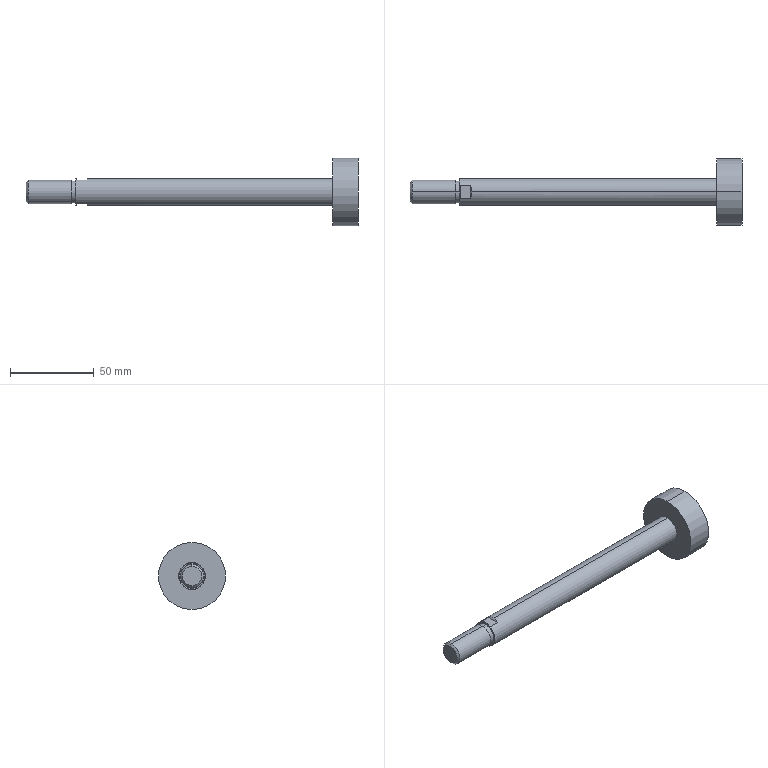Part | SolidWorks | features BaseBody 1 | 1 solid | 23 faces | box 198 x 40 x 40 mm | volume 54072 mm3 | plane 11 | cylinder 8 | cone 4 | commonest cylinder face diameters 13 x2 14 x2 16 x2 40 x2
STEP:
#1=CARTESIAN_POINT('',(133.,0.,8.));
#2=VERTEX_POINT('',#1);
#3=CARTESIAN_POINT('',(133.,0.,-8.));
#4=VERTEX_POINT('',#3);
#5=CARTESIAN_POINT('',(133.,0.,0.));
#6=DIRECTION('',(-1.,0.,0.));
#7=DIRECTION('',(0.,0.,1.));
#8=AXIS2_PLACEMENT_3D('',#5,#6,#7);
#9=CIRCLE('',#8,8.);
#10=EDGE_CURVE('',#2,#4,#9,.T.);
#11=ORIENTED_EDGE('',*,*,#10,.T.);
#12=CARTESIAN_POINT('',(-13.,0.,-8.));
#13=VERTEX_POINT('',#12);
#14=CARTESIAN_POINT('',(148.,0.,-8.));
#15=DIRECTION('',(-1.,0.,0.));
#16=VECTOR('',#15,1000.);
#17=LINE('',#14,#16);
#18=EDGE_CURVE('',#4,#13,#17,.T.);
#19=ORIENTED_EDGE('',*,*,#18,.T.);
#20=CARTESIAN_POINT('',(-14.,3.873,-7.));
#21=VERTEX_POINT('',#20);
#22=CARTESIAN_POINT('',(-13.,0.,-8.));
#23=CARTESIAN_POINT('',(-13.,1.362,-8.));
#24=CARTESIAN_POINT('',(-13.341,2.681,-7.659));
#25=CARTESIAN_POINT('',(-14.,3.873,-7.));
#26=(BOUNDED_CURVE()B_SPLINE_CURVE(3,(#22,#23,#24,#25),.UNSPECIFIED.,.F.,.F.)B_SPLINE_CURVE_WITH_KNOTS((4,4),(3.142,3.647),.UNSPECIFIED.)CURVE()GEOMETRIC_REPRESENTATION_ITEM()RATIONAL_B_SPLINE_CURVE((1.,0.9788,0.9788,1.))REPRESENTATION_ITEM(''));
#27=EDGE_CURVE('',#13,#21,#26,.T.);
#28=ORIENTED_EDGE('',*,*,#27,.T.);
#29=CARTESIAN_POINT('',(-20.,3.873,-7.));
#30=VERTEX_POINT('',#29);
#31=CARTESIAN_POINT('',(148.,3.873,-7.));
#32=DIRECTION('',(-1.,0.,0.));
#33=VECTOR('',#32,1000.);
#34=LINE('',#31,#33);
#35=EDGE_CURVE('',#21,#30,#34,.T.);
#36=ORIENTED_EDGE('',*,*,#35,.T.);
#37=CARTESIAN_POINT('',(-20.,0.,-8.));
#38=VERTEX_POINT('',#37);
#39=CARTESIAN_POINT('',(-20.,0.,0.));
#40=DIRECTION('',(-1.,0.,0.));
#41=DIRECTION('',(0.,0.,1.));
#42=AXIS2_PLACEMENT_3D('',#39,#40,#41);
#43=CIRCLE('',#42,8.);
#44=EDGE_CURVE('',#30,#38,#43,.T.);
#45=ORIENTED_EDGE('',*,*,#44,.T.);
#46=CARTESIAN_POINT('',(-20.4,0.,-8.));
#47=VERTEX_POINT('',#46);
#48=CARTESIAN_POINT('',(148.,0.,-8.));
#49=DIRECTION('',(-1.,0.,0.));
#50=VECTOR('',#49,1000.);
#51=LINE('',#48,#50);
#52=EDGE_CURVE('',#38,#47,#51,.T.);
#53=ORIENTED_EDGE('',*,*,#52,.T.);
#54=CARTESIAN_POINT('',(-20.4,0.,8.));
#55=VERTEX_POINT('',#54);
#56=CARTESIAN_POINT('',(-20.4,0.,0.));
#57=DIRECTION('',(1.,0.,0.));
#58=DIRECTION('',(0.,0.,1.));
#59=AXIS2_PLACEMENT_3D('',#56,#57,#58);
#60=CIRCLE('',#59,8.);
#61=EDGE_CURVE('',#47,#55,#60,.T.);
#62=ORIENTED_EDGE('',*,*,#61,.T.);
#63=CARTESIAN_POINT('',(-20.,0.,8.));
#64=VERTEX_POINT('',#63);
#65=CARTESIAN_POINT('',(148.,0.,8.));
#66=DIRECTION('',(-1.,0.,0.));
#67=VECTOR('',#66,1000.);
#68=LINE('',#65,#67);
#69=EDGE_CURVE('',#64,#55,#68,.T.);
#70=ORIENTED_EDGE('',*,*,#69,.F.);
#71=CARTESIAN_POINT('',(-20.,3.873,7.));
#72=VERTEX_POINT('',#71);
#73=CARTESIAN_POINT('',(-20.,0.,0.));
#74=DIRECTION('',(-1.,0.,0.));
#75=DIRECTION('',(0.,0.,1.));
#76=AXIS2_PLACEMENT_3D('',#73,#74,#75);
#77=CIRCLE('',#76,8.);
#78=EDGE_CURVE('',#64,#72,#77,.T.);
#79=ORIENTED_EDGE('',*,*,#78,.T.);
#80=CARTESIAN_POINT('',(-14.,3.873,7.));
#81=VERTEX_POINT('',#80);
#82=CARTESIAN_POINT('',(148.,3.873,7.));
#83=DIRECTION('',(1.,0.,0.));
#84=VECTOR('',#83,1000.);
#85=LINE('',#82,#84);
#86=EDGE_CURVE('',#72,#81,#85,.T.);
#87=ORIENTED_EDGE('',*,*,#86,.T.);
#88=CARTESIAN_POINT('',(-13.,0.,8.));
#89=VERTEX_POINT('',#88);
#90=CARTESIAN_POINT('',(-14.,3.873,7.));
#91=CARTESIAN_POINT('',(-13.341,2.681,7.659));
#92=CARTESIAN_POINT('',(-13.,1.362,8.));
#93=CARTESIAN_POINT('',(-13.,0.,8.));
#94=(BOUNDED_CURVE()B_SPLINE_CURVE(3,(#90,#91,#92,#93),.UNSPECIFIED.,.F.,.T.)B_SPLINE_CURVE_WITH_KNOTS((4,4),(2.636,3.142),.UNSPECIFIED.)CURVE()GEOMETRIC_REPRESENTATION_ITEM()RATIONAL_B_SPLINE_CURVE((1.,0.9788,0.9788,1.))REPRESENTATION_ITEM(''));
#95=EDGE_CURVE('',#81,#89,#94,.T.);
#96=ORIENTED_EDGE('',*,*,#95,.T.);
#97=CARTESIAN_POINT('',(148.,0.,8.));
#98=DIRECTION('',(-1.,0.,0.));
#99=VECTOR('',#98,1000.);
#100=LINE('',#97,#99);
#101=EDGE_CURVE('',#2,#89,#100,.T.);
#102=ORIENTED_EDGE('',*,*,#101,.F.);
#103=EDGE_LOOP('',(#11,#19,#28,#36,#45,#53,#62,#70,#79,#87,#96,#102));
#104=FACE_OUTER_BOUND('',#103,.T.);
#105=CARTESIAN_POINT('',(148.,0.,0.));
#106=DIRECTION('',(-1.,0.,0.));
#107=DIRECTION('',(0.,0.,1.));
#108=AXIS2_PLACEMENT_3D('',#105,#106,#107);
#109=CYLINDRICAL_SURFACE('',#108,8.);
#110=ADVANCED_FACE('',(#104),#109,.T.);
#111=CARTESIAN_POINT('',(-20.,0.,-7.6));
#112=VERTEX_POINT('',#111);
#113=CARTESIAN_POINT('',(-20.,-2.96,-7.));
#114=VERTEX_POINT('',#113);
#115=CARTESIAN_POINT('',(-20.,0.,0.));
#116=DIRECTION('',(-1.,0.,0.));
#117=DIRECTION('',(0.,0.,1.));
#118=AXIS2_PLACEMENT_3D('',#115,#116,#117);
#119=CIRCLE('',#118,7.6);
#120=EDGE_CURVE('',#112,#114,#119,.T.);
#121=ORIENTED_EDGE('',*,*,#120,.F.);
#122=CARTESIAN_POINT('',(-20.4,0.,-8.));
#123=DIRECTION('',(-0.7071,0.,-0.7071));
#124=VECTOR('',#123,1000.);
#125=LINE('',#122,#124);
#126=EDGE_CURVE('',#112,#47,#125,.T.);
#127=ORIENTED_EDGE('',*,*,#126,.T.);
#128=CARTESIAN_POINT('',(-20.4,0.,0.));
#129=DIRECTION('',(1.,0.,0.));
#130=DIRECTION('',(0.,0.,1.));
#131=AXIS2_PLACEMENT_3D('',#128,#129,#130);
#132=CIRCLE('',#131,8.);
#133=EDGE_CURVE('',#55,#47,#132,.T.);
#134=ORIENTED_EDGE('',*,*,#133,.F.);
#135=CARTESIAN_POINT('',(-20.,0.,7.6));
#136=VERTEX_POINT('',#135);
#137=CARTESIAN_POINT('',(-20.4,0.,8.));
#138=DIRECTION('',(-0.7071,0.,0.7071));
#139=VECTOR('',#138,1000.);
#140=LINE('',#137,#139);
#141=EDGE_CURVE('',#136,#55,#140,.T.);
#142=ORIENTED_EDGE('',*,*,#141,.F.);
#143=CARTESIAN_POINT('',(-20.,-2.96,7.));
#144=VERTEX_POINT('',#143);
#145=CARTESIAN_POINT('',(-20.,0.,0.));
#146=DIRECTION('',(-1.,0.,0.));
#147=DIRECTION('',(0.,0.,1.));
#148=AXIS2_PLACEMENT_3D('',#145,#146,#147);
#149=CIRCLE('',#148,7.6);
#150=EDGE_CURVE('',#144,#136,#149,.T.);
#151=ORIENTED_EDGE('',*,*,#150,.F.);
#152=CARTESIAN_POINT('',(-20.,0.,0.));
#153=DIRECTION('',(-1.,0.,0.));
#154=DIRECTION('',(0.,0.,1.));
#155=AXIS2_PLACEMENT_3D('',#152,#153,#154);
#156=CIRCLE('',#155,7.6);
#157=EDGE_CURVE('',#114,#144,#156,.T.);
#158=ORIENTED_EDGE('',*,*,#157,.F.);
#159=EDGE_LOOP('',(#121,#127,#134,#142,#151,#158));
#160=FACE_OUTER_BOUND('',#159,.T.);
#161=CARTESIAN_POINT('',(-20.4,0.,0.));
#162=DIRECTION('',(-1.,0.,0.));
#163=DIRECTION('',(0.,0.,1.));
#164=AXIS2_PLACEMENT_3D('',#161,#162,#163);
#165=CONICAL_SURFACE('',#164,8.,0.7854);
#166=ADVANCED_FACE('',(#160),#165,.F.);
#167=CARTESIAN_POINT('',(148.,0.,20.));
#168=VERTEX_POINT('',#167);
#169=CARTESIAN_POINT('',(148.,0.,-20.));
#170=VERTEX_POINT('',#169);
#171=CARTESIAN_POINT('',(148.,0.,0.));
#172=DIRECTION('',(-1.,0.,0.));
#173=DIRECTION('',(0.,0.,1.));
#174=AXIS2_PLACEMENT_3D('',#171,#172,#173);
#175=CIRCLE('',#174,20.);
#176=EDGE_CURVE('',#168,#170,#175,.T.);
#177=ORIENTED_EDGE('',*,*,#176,.T.);
#178=CARTESIAN_POINT('',(133.,0.,-20.));
#179=VERTEX_POINT('',#178);
#180=CARTESIAN_POINT('',(148.,0.,-20.));
#181=DIRECTION('',(-1.,0.,0.));
#182=VECTOR('',#181,1000.);
#183=LINE('',#180,#182);
#184=EDGE_CURVE('',#170,#179,#183,.T.);
#185=ORIENTED_EDGE('',*,*,#184,.T.);
#186=CARTESIAN_POINT('',(133.,0.,20.));
#187=VERTEX_POINT('',#186);
#188=CARTESIAN_POINT('',(133.,0.,0.));
#189=DIRECTION('',(1.,0.,0.));
#190=DIRECTION('',(0.,0.,1.));
#191=AXIS2_PLACEMENT_3D('',#188,#189,#190);
#192=CIRCLE('',#191,20.);
#193=EDGE_CURVE('',#179,#187,#192,.T.);
#194=ORIENTED_EDGE('',*,*,#193,.T.);
#195=CARTESIAN_POINT('',(148.,0.,20.));
#196=DIRECTION('',(-1.,0.,0.));
#197=VECTOR('',#196,1000.);
#198=LINE('',#195,#197);
#199=EDGE_CURVE('',#168,#187,#198,.T.);
#200=ORIENTED_EDGE('',*,*,#199,.F.);
#201=EDGE_LOOP('',(#177,#185,#194,#200));
#202=FACE_OUTER_BOUND('',#201,.T.);
#203=CARTESIAN_POINT('',(148.,0.,0.));
#204=DIRECTION('',(-1.,0.,0.));
#205=DIRECTION('',(0.,0.,1.));
#206=AXIS2_PLACEMENT_3D('',#203,#204,#205);
#207=CYLINDRICAL_SURFACE('',#206,20.);
#208=ADVANCED_FACE('',(#202),#207,.T.);
#209=CARTESIAN_POINT('',(-20.,0.,6.5));
#210=VERTEX_POINT('',#209);
#211=CARTESIAN_POINT('',(-20.,0.,-6.5));
#212=VERTEX_POINT('',#211);
#213=CARTESIAN_POINT('',(-20.,0.,0.));
#214=DIRECTION('',(-1.,0.,0.));
#215=DIRECTION('',(0.,0.,1.));
#216=AXIS2_PLACEMENT_3D('',#213,#214,#215);
#217=CIRCLE('',#216,6.5);
#218=EDGE_CURVE('',#210,#212,#217,.T.);
#219=ORIENTED_EDGE('',*,*,#218,.T.);
#220=CARTESIAN_POINT('',(-23.,0.,-6.5));
#221=VERTEX_POINT('',#220);
#222=CARTESIAN_POINT('',(148.,0.,-6.5));
#223=DIRECTION('',(-1.,0.,0.));
#224=VECTOR('',#223,1000.);
#225=LINE('',#222,#224);
#226=EDGE_CURVE('',#212,#221,#225,.T.);
#227=ORIENTED_EDGE('',*,*,#226,.T.);
#228=CARTESIAN_POINT('',(-23.,0.,6.5));
#229=VERTEX_POINT('',#228);
#230=CARTESIAN_POINT('',(-23.,0.,0.));
#231=DIRECTION('',(1.,0.,0.));
#232=DIRECTION('',(0.,0.,1.));
#233=AXIS2_PLACEMENT_3D('',#230,#231,#232);
#234=CIRCLE('',#233,6.5);
#235=EDGE_CURVE('',#221,#229,#234,.T.);
#236=ORIENTED_EDGE('',*,*,#235,.T.);
#237=CARTESIAN_POINT('',(148.,0.,6.5));
#238=DIRECTION('',(-1.,0.,0.));
#239=VECTOR('',#238,1000.);
#240=LINE('',#237,#239);
#241=EDGE_CURVE('',#210,#229,#240,.T.);
#242=ORIENTED_EDGE('',*,*,#241,.F.);
#243=EDGE_LOOP('',(#219,#227,#236,#242));
#244=FACE_OUTER_BOUND('',#243,.T.);
#245=CARTESIAN_POINT('',(148.,0.,0.));
#246=DIRECTION('',(-1.,0.,0.));
#247=DIRECTION('',(0.,0.,1.));
#248=AXIS2_PLACEMENT_3D('',#245,#246,#247);
#249=CYLINDRICAL_SURFACE('',#248,6.5);
#250=ADVANCED_FACE('',(#244),#249,.T.);
#251=CARTESIAN_POINT('',(-23.,0.,7.));
#252=VERTEX_POINT('',#251);
#253=CARTESIAN_POINT('',(-23.,0.,-7.));
#254=VERTEX_POINT('',#253);
#255=CARTESIAN_POINT('',(-23.,0.,0.));
#256=DIRECTION('',(-1.,0.,0.));
#257=DIRECTION('',(0.,0.,1.));
#258=AXIS2_PLACEMENT_3D('',#255,#256,#257);
#259=CIRCLE('',#258,7.);
#260=EDGE_CURVE('',#252,#254,#259,.T.);
#261=ORIENTED_EDGE('',*,*,#260,.T.);
#262=CARTESIAN_POINT('',(-48.773,0.,-7.));
#263=VERTEX_POINT('',#262);
#264=CARTESIAN_POINT('',(148.,0.,-7.));
#265=DIRECTION('',(-1.,0.,0.));
#266=VECTOR('',#265,1000.);
#267=LINE('',#264,#266);
#268=EDGE_CURVE('',#254,#263,#267,.T.);
#269=ORIENTED_EDGE('',*,*,#268,.T.);
#270=CARTESIAN_POINT('',(-48.773,0.,7.));
#271=VERTEX_POINT('',#270);
#272=CARTESIAN_POINT('',(-48.773,0.,0.));
#273=DIRECTION('',(1.,0.,0.));
#274=DIRECTION('',(0.,0.,1.));
#275=AXIS2_PLACEMENT_3D('',#272,#273,#274);
#276=CIRCLE('',#275,7.);
#277=EDGE_CURVE('',#263,#271,#276,.T.);
#278=ORIENTED_EDGE('',*,*,#277,.T.);
#279=CARTESIAN_POINT('',(148.,0.,7.));
#280=DIRECTION('',(-1.,0.,0.));
#281=VECTOR('',#280,1000.);
#282=LINE('',#279,#281);
#283=EDGE_CURVE('',#252,#271,#282,.T.);
#284=ORIENTED_EDGE('',*,*,#283,.F.);
#285=EDGE_LOOP('',(#261,#269,#278,#284));
#286=FACE_OUTER_BOUND('',#285,.T.);
#287=CARTESIAN_POINT('',(148.,0.,0.));
#288=DIRECTION('',(-1.,0.,0.));
#289=DIRECTION('',(0.,0.,1.));
#290=AXIS2_PLACEMENT_3D('',#287,#288,#289);
#291=CYLINDRICAL_SURFACE('',#290,7.);
#292=ADVANCED_FACE('',(#286),#291,.T.);
#293=CARTESIAN_POINT('',(-50.,0.,-5.773));
#294=VERTEX_POINT('',#293);
#295=CARTESIAN_POINT('',(-50.,0.,5.773));
#296=VERTEX_POINT('',#295);
#297=CARTESIAN_POINT('',(-50.,0.,0.));
#298=DIRECTION('',(1.,0.,0.));
#299=DIRECTION('',(0.,0.,-1.));
#300=AXIS2_PLACEMENT_3D('',#297,#298,#299);
#301=CIRCLE('',#300,5.773);
#302=EDGE_CURVE('',#294,#296,#301,.T.);
#303=ORIENTED_EDGE('',*,*,#302,.T.);
#304=CARTESIAN_POINT('',(-48.773,0.,7.));
#305=DIRECTION('',(0.7071,0.,0.7071));
#306=VECTOR('',#305,1000.);
#307=LINE('',#304,#306);
#308=EDGE_CURVE('',#296,#271,#307,.T.);
#309=ORIENTED_EDGE('',*,*,#308,.T.);
#310=ORIENTED_EDGE('',*,*,#277,.F.);
#311=CARTESIAN_POINT('',(-48.773,0.,-7.));
#312=DIRECTION('',(0.7071,0.,-0.7071));
#313=VECTOR('',#312,1000.);
#314=LINE('',#311,#313);
#315=EDGE_CURVE('',#294,#263,#314,.T.);
#316=ORIENTED_EDGE('',*,*,#315,.F.);
#317=EDGE_LOOP('',(#303,#309,#310,#316));
#318=FACE_OUTER_BOUND('',#317,.T.);
#319=CARTESIAN_POINT('',(-48.773,0.,0.));
#320=DIRECTION('',(1.,0.,0.));
#321=DIRECTION('',(0.,0.,-1.));
#322=AXIS2_PLACEMENT_3D('',#319,#320,#321);
#323=CONICAL_SURFACE('',#322,7.,0.7854);
#324=ADVANCED_FACE('',(#318),#323,.T.);
#325=ORIENTED_EDGE('',*,*,#18,.F.);
#326=CARTESIAN_POINT('',(133.,0.,0.));
#327=DIRECTION('',(-1.,0.,0.));
#328=DIRECTION('',(0.,0.,1.));
#329=AXIS2_PLACEMENT_3D('',#326,#327,#328);
#330=CIRCLE('',#329,8.);
#331=EDGE_CURVE('',#4,#2,#330,.T.);
#332=ORIENTED_EDGE('',*,*,#331,.T.);
#333=ORIENTED_EDGE('',*,*,#101,.T.);
#334=CARTESIAN_POINT('',(-14.,-3.873,7.));
#335=VERTEX_POINT('',#334);
#336=CARTESIAN_POINT('',(-13.,0.,8.));
#337=CARTESIAN_POINT('',(-13.,-1.362,8.));
#338=CARTESIAN_POINT('',(-13.341,-2.681,7.659));
#339=CARTESIAN_POINT('',(-14.,-3.873,7.));
#340=(BOUNDED_CURVE()B_SPLINE_CURVE(3,(#336,#337,#338,#339),.UNSPECIFIED.,.F.,.F.)B_SPLINE_CURVE_WITH_KNOTS((4,4),(3.142,3.647),.UNSPECIFIED.)CURVE()GEOMETRIC_REPRESENTATION_ITEM()RATIONAL_B_SPLINE_CURVE((1.,0.9788,0.9788,1.))REPRESENTATION_ITEM(''));
#341=EDGE_CURVE('',#89,#335,#340,.T.);
#342=ORIENTED_EDGE('',*,*,#341,.T.);
#343=CARTESIAN_POINT('',(-20.,-3.873,7.));
#344=VERTEX_POINT('',#343);
#345=CARTESIAN_POINT('',(148.,-3.873,7.));
#346=DIRECTION('',(-1.,0.,0.));
#347=VECTOR('',#346,1000.);
#348=LINE('',#345,#347);
#349=EDGE_CURVE('',#335,#344,#348,.T.);
#350=ORIENTED_EDGE('',*,*,#349,.T.);
#351=CARTESIAN_POINT('',(-20.,0.,0.));
#352=DIRECTION('',(-1.,0.,0.));
#353=DIRECTION('',(0.,0.,1.));
#354=AXIS2_PLACEMENT_3D('',#351,#352,#353);
#355=CIRCLE('',#354,8.);
#356=EDGE_CURVE('',#344,#64,#355,.T.);
#357=ORIENTED_EDGE('',*,*,#356,.T.);
#358=ORIENTED_EDGE('',*,*,#69,.T.);
#359=ORIENTED_EDGE('',*,*,#133,.T.);
#360=ORIENTED_EDGE('',*,*,#52,.F.);
#361=CARTESIAN_POINT('',(-20.,-3.873,-7.));
#362=VERTEX_POINT('',#361);
#363=CARTESIAN_POINT('',(-20.,0.,0.));
#364=DIRECTION('',(-1.,0.,0.));
#365=DIRECTION('',(0.,0.,1.));
#366=AXIS2_PLACEMENT_3D('',#363,#364,#365);
#367=CIRCLE('',#366,8.);
#368=EDGE_CURVE('',#38,#362,#367,.T.);
#369=ORIENTED_EDGE('',*,*,#368,.T.);
#370=CARTESIAN_POINT('',(-14.,-3.873,-7.));
#371=VERTEX_POINT('',#370);
#372=CARTESIAN_POINT('',(148.,-3.873,-7.));
#373=DIRECTION('',(1.,0.,0.));
#374=VECTOR('',#373,1000.);
#375=LINE('',#372,#374);
#376=EDGE_CURVE('',#362,#371,#375,.T.);
#377=ORIENTED_EDGE('',*,*,#376,.T.);
#378=CARTESIAN_POINT('',(-14.,-3.873,-7.));
#379=CARTESIAN_POINT('',(-13.341,-2.681,-7.659));
#380=CARTESIAN_POINT('',(-13.,-1.362,-8.));
#381=CARTESIAN_POINT('',(-13.,0.,-8.));
#382=(BOUNDED_CURVE()B_SPLINE_CURVE(3,(#378,#379,#380,#381),.UNSPECIFIED.,.F.,.F.)B_SPLINE_CURVE_WITH_KNOTS((4,4),(2.636,3.142),.UNSPECIFIED.)CURVE()GEOMETRIC_REPRESENTATION_ITEM()RATIONAL_B_SPLINE_CURVE((1.,0.9788,0.9788,1.))REPRESENTATION_ITEM(''));
#383=EDGE_CURVE('',#371,#13,#382,.T.);
#384=ORIENTED_EDGE('',*,*,#383,.T.);
#385=EDGE_LOOP('',(#325,#332,#333,#342,#350,#357,#358,#359,#360,#369,#377,#384));
#386=FACE_OUTER_BOUND('',#385,.T.);
#387=CARTESIAN_POINT('',(148.,0.,0.));
#388=DIRECTION('',(-1.,0.,0.));
#389=DIRECTION('',(0.,0.,1.));
#390=AXIS2_PLACEMENT_3D('',#387,#388,#389);
#391=CYLINDRICAL_SURFACE('',#390,8.);
#392=ADVANCED_FACE('',(#386),#391,.T.);
#393=CARTESIAN_POINT('',(-20.,2.96,7.));
#394=VERTEX_POINT('',#393);
#395=CARTESIAN_POINT('',(-20.,8.,7.));
#396=DIRECTION('',(0.,-1.,0.));
#397=VECTOR('',#396,1000.);
#398=LINE('',#395,#397);
#399=EDGE_CURVE('',#394,#144,#398,.T.);
#400=ORIENTED_EDGE('',*,*,#399,.T.);
#401=CARTESIAN_POINT('',(-20.,8.,7.));
#402=DIRECTION('',(0.,-1.,0.));
#403=VECTOR('',#402,1000.);
#404=LINE('',#401,#403);
#405=EDGE_CURVE('',#144,#344,#404,.T.);
#406=ORIENTED_EDGE('',*,*,#405,.T.);
#407=ORIENTED_EDGE('',*,*,#349,.F.);
#408=CARTESIAN_POINT('',(-14.,8.,7.));
#409=DIRECTION('',(0.,1.,0.));
#410=VECTOR('',#409,1000.);
#411=LINE('',#408,#410);
#412=EDGE_CURVE('',#335,#81,#411,.T.);
#413=ORIENTED_EDGE('',*,*,#412,.T.);
#414=ORIENTED_EDGE('',*,*,#86,.F.);
#415=CARTESIAN_POINT('',(-20.,8.,7.));
#416=DIRECTION('',(0.,-1.,0.));
#417=VECTOR('',#416,1000.);
#418=LINE('',#415,#417);
#419=EDGE_CURVE('',#72,#394,#418,.T.);
#420=ORIENTED_EDGE('',*,*,#419,.T.);
#421=EDGE_LOOP('',(#400,#406,#407,#413,#414,#420));
#422=FACE_OUTER_BOUND('',#421,.T.);
#423=CARTESIAN_POINT('',(-14.,8.,7.));
#424=DIRECTION('',(0.,0.,1.));
#425=DIRECTION('',(1.,0.,0.));
#426=AXIS2_PLACEMENT_3D('',#423,#424,#425);
#427=PLANE('',#426);
#428=ADVANCED_FACE('',(#422),#427,.T.);
#429=ORIENTED_EDGE('',*,*,#356,.F.);
#430=ORIENTED_EDGE('',*,*,#405,.F.);
#431=ORIENTED_EDGE('',*,*,#150,.T.);
#432=CARTESIAN_POINT('',(-20.,0.,0.));
#433=DIRECTION('',(-1.,0.,0.));
#434=DIRECTION('',(0.,0.,1.));
#435=AXIS2_PLACEMENT_3D('',#432,#433,#434);
#436=CIRCLE('',#435,7.6);
#437=EDGE_CURVE('',#136,#394,#436,.T.);
#438=ORIENTED_EDGE('',*,*,#437,.T.);
#439=ORIENTED_EDGE('',*,*,#419,.F.);
#440=ORIENTED_EDGE('',*,*,#78,.F.);
#441=EDGE_LOOP('',(#429,#430,#431,#438,#439,#440));
#442=FACE_OUTER_BOUND('',#441,.T.);
#443=CARTESIAN_POINT('',(-20.,8.,7.));
#444=DIRECTION('',(1.,0.,0.));
#445=DIRECTION('',(0.,0.,-1.));
#446=AXIS2_PLACEMENT_3D('',#443,#444,#445);
#447=PLANE('',#446);
#448=ADVANCED_FACE('',(#442),#447,.T.);
#449=ORIENTED_EDGE('',*,*,#95,.F.);
#450=ORIENTED_EDGE('',*,*,#412,.F.);
#451=ORIENTED_EDGE('',*,*,#341,.F.);
#452=EDGE_LOOP('',(#449,#450,#451));
#453=FACE_OUTER_BOUND('',#452,.T.);
#454=CARTESIAN_POINT('',(-5.,8.,16.));
#455=DIRECTION('',(-0.7071,0.,0.7071));
#456=DIRECTION('',(0.7071,0.,0.7071));
#457=AXIS2_PLACEMENT_3D('',#454,#455,#456);
#458=PLANE('',#457);
#459=ADVANCED_FACE('',(#453),#458,.T.);
#460=ORIENTED_EDGE('',*,*,#126,.F.);
#461=CARTESIAN_POINT('',(-20.,2.96,-7.));
#462=VERTEX_POINT('',#461);
#463=CARTESIAN_POINT('',(-20.,0.,0.));
#464=DIRECTION('',(-1.,0.,0.));
#465=DIRECTION('',(0.,0.,1.));
#466=AXIS2_PLACEMENT_3D('',#463,#464,#465);
#467=CIRCLE('',#466,7.6);
#468=EDGE_CURVE('',#462,#112,#467,.T.);
#469=ORIENTED_EDGE('',*,*,#468,.F.);
#470=CARTESIAN_POINT('',(-20.,0.,0.));
#471=DIRECTION('',(-1.,0.,0.));
#472=DIRECTION('',(0.,0.,1.));
#473=AXIS2_PLACEMENT_3D('',#470,#471,#472);
#474=CIRCLE('',#473,7.6);
#475=EDGE_CURVE('',#394,#462,#474,.T.);
#476=ORIENTED_EDGE('',*,*,#475,.F.);
#477=ORIENTED_EDGE('',*,*,#437,.F.);
#478=ORIENTED_EDGE('',*,*,#141,.T.);
#479=ORIENTED_EDGE('',*,*,#61,.F.);
#480=EDGE_LOOP('',(#460,#469,#476,#477,#478,#479));
#481=FACE_OUTER_BOUND('',#480,.T.);
#482=CARTESIAN_POINT('',(-20.4,0.,0.));
#483=DIRECTION('',(-1.,0.,0.));
#484=DIRECTION('',(0.,0.,1.));
#485=AXIS2_PLACEMENT_3D('',#482,#483,#484);
#486=CONICAL_SURFACE('',#485,8.,0.7854);
#487=ADVANCED_FACE('',(#481),#486,.F.);
#488=CARTESIAN_POINT('',(-20.,8.,-7.));
#489=DIRECTION('',(0.,1.,0.));
#490=VECTOR('',#489,1000.);
#491=LINE('',#488,#490);
#492=EDGE_CURVE('',#114,#462,#491,.T.);
#493=ORIENTED_EDGE('',*,*,#492,.T.);
#494=CARTESIAN_POINT('',(-20.,8.,-7.));
#495=DIRECTION('',(0.,1.,0.));
#496=VECTOR('',#495,1000.);
#497=LINE('',#494,#496);
#498=EDGE_CURVE('',#462,#30,#497,.T.);
#499=ORIENTED_EDGE('',*,*,#498,.T.);
#500=ORIENTED_EDGE('',*,*,#35,.F.);
#501=CARTESIAN_POINT('',(-14.,8.,-7.));
#502=DIRECTION('',(0.,-1.,0.));
#503=VECTOR('',#502,1000.);
#504=LINE('',#501,#503);
#505=EDGE_CURVE('',#21,#371,#504,.T.);
#506=ORIENTED_EDGE('',*,*,#505,.T.);
#507=ORIENTED_EDGE('',*,*,#376,.F.);
#508=CARTESIAN_POINT('',(-20.,8.,-7.));
#509=DIRECTION('',(0.,1.,0.));
#510=VECTOR('',#509,1000.);
#511=LINE('',#508,#510);
#512=EDGE_CURVE('',#362,#114,#511,.T.);
#513=ORIENTED_EDGE('',*,*,#512,.T.);
#514=EDGE_LOOP('',(#493,#499,#500,#506,#507,#513));
#515=FACE_OUTER_BOUND('',#514,.T.);
#516=CARTESIAN_POINT('',(-20.,8.,-7.));
#517=DIRECTION('',(0.,0.,-1.));
#518=DIRECTION('',(-1.,0.,0.));
#519=AXIS2_PLACEMENT_3D('',#516,#517,#518);
#520=PLANE('',#519);
#521=ADVANCED_FACE('',(#515),#520,.T.);
#522=ORIENTED_EDGE('',*,*,#383,.F.);
#523=ORIENTED_EDGE('',*,*,#505,.F.);
#524=ORIENTED_EDGE('',*,*,#27,.F.);
#525=EDGE_LOOP('',(#522,#523,#524));
#526=FACE_OUTER_BOUND('',#525,.T.);
#527=CARTESIAN_POINT('',(-14.,8.,-7.));
#528=DIRECTION('',(-0.7071,0.,-0.7071));
#529=DIRECTION('',(-0.7071,0.,0.7071));
#530=AXIS2_PLACEMENT_3D('',#527,#528,#529);
#531=PLANE('',#530);
#532=ADVANCED_FACE('',(#526),#531,.T.);
#533=ORIENTED_EDGE('',*,*,#44,.F.);
#534=ORIENTED_EDGE('',*,*,#498,.F.);
#535=ORIENTED_EDGE('',*,*,#468,.T.);
#536=ORIENTED_EDGE('',*,*,#120,.T.);
#537=ORIENTED_EDGE('',*,*,#512,.F.);
#538=ORIENTED_EDGE('',*,*,#368,.F.);
#539=EDGE_LOOP('',(#533,#534,#535,#536,#537,#538));
#540=FACE_OUTER_BOUND('',#539,.T.);
#541=CARTESIAN_POINT('',(-20.,8.,-13.6));
#542=DIRECTION('',(1.,0.,0.));
#543=DIRECTION('',(0.,0.,-1.));
#544=AXIS2_PLACEMENT_3D('',#541,#542,#543);
#545=PLANE('',#544);
#546=ADVANCED_FACE('',(#540),#545,.T.);
#547=ORIENTED_EDGE('',*,*,#10,.F.);
#548=ORIENTED_EDGE('',*,*,#331,.F.);
#549=EDGE_LOOP('',(#547,#548));
#550=FACE_BOUND('',#549,.T.);
#551=CARTESIAN_POINT('',(133.,0.,0.));
#552=DIRECTION('',(1.,0.,0.));
#553=DIRECTION('',(0.,0.,1.));
#554=AXIS2_PLACEMENT_3D('',#551,#552,#553);
#555=CIRCLE('',#554,20.);
#556=EDGE_CURVE('',#187,#179,#555,.T.);
#557=ORIENTED_EDGE('',*,*,#556,.F.);
#558=ORIENTED_EDGE('',*,*,#193,.F.);
#559=EDGE_LOOP('',(#557,#558));
#560=FACE_OUTER_BOUND('',#559,.T.);
#561=CARTESIAN_POINT('',(133.,8.,0.));
#562=DIRECTION('',(1.,0.,0.));
#563=DIRECTION('',(0.,0.,-1.));
#564=AXIS2_PLACEMENT_3D('',#561,#562,#563);
#565=PLANE('',#564);
#566=ADVANCED_FACE('',(#550,#560),#565,.F.);
#567=ORIENTED_EDGE('',*,*,#218,.F.);
#568=CARTESIAN_POINT('',(-20.,0.,0.));
#569=DIRECTION('',(-1.,0.,0.));
#570=DIRECTION('',(0.,0.,1.));
#571=AXIS2_PLACEMENT_3D('',#568,#569,#570);
#572=CIRCLE('',#571,6.5);
#573=EDGE_CURVE('',#212,#210,#572,.T.);
#574=ORIENTED_EDGE('',*,*,#573,.F.);
#575=EDGE_LOOP('',(#567,#574));
#576=FACE_BOUND('',#575,.T.);
#577=ORIENTED_EDGE('',*,*,#492,.F.);
#578=ORIENTED_EDGE('',*,*,#157,.T.);
#579=ORIENTED_EDGE('',*,*,#399,.F.);
#580=ORIENTED_EDGE('',*,*,#475,.T.);
#581=EDGE_LOOP('',(#577,#578,#579,#580));
#582=FACE_OUTER_BOUND('',#581,.T.);
#583=CARTESIAN_POINT('',(-20.,6.5,0.));
#584=DIRECTION('',(1.,0.,0.));
#585=DIRECTION('',(0.,0.,-1.));
#586=AXIS2_PLACEMENT_3D('',#583,#584,#585);
#587=PLANE('',#586);
#588=ADVANCED_FACE('',(#576,#582),#587,.F.);
#589=ORIENTED_EDGE('',*,*,#184,.F.);
#590=CARTESIAN_POINT('',(148.,0.,0.));
#591=DIRECTION('',(-1.,0.,0.));
#592=DIRECTION('',(0.,0.,1.));
#593=AXIS2_PLACEMENT_3D('',#590,#591,#592);
#594=CIRCLE('',#593,20.);
#595=EDGE_CURVE('',#170,#168,#594,.T.);
#596=ORIENTED_EDGE('',*,*,#595,.T.);
#597=ORIENTED_EDGE('',*,*,#199,.T.);
#598=ORIENTED_EDGE('',*,*,#556,.T.);
#599=EDGE_LOOP('',(#589,#596,#597,#598));
#600=FACE_OUTER_BOUND('',#599,.T.);
#601=CARTESIAN_POINT('',(148.,0.,0.));
#602=DIRECTION('',(-1.,0.,0.));
#603=DIRECTION('',(0.,0.,1.));
#604=AXIS2_PLACEMENT_3D('',#601,#602,#603);
#605=CYLINDRICAL_SURFACE('',#604,20.);
#606=ADVANCED_FACE('',(#600),#605,.T.);
#607=ORIENTED_EDGE('',*,*,#226,.F.);
#608=ORIENTED_EDGE('',*,*,#573,.T.);
#609=ORIENTED_EDGE('',*,*,#241,.T.);
#610=CARTESIAN_POINT('',(-23.,0.,0.));
#611=DIRECTION('',(1.,0.,0.));
#612=DIRECTION('',(0.,0.,1.));
#613=AXIS2_PLACEMENT_3D('',#610,#611,#612);
#614=CIRCLE('',#613,6.5);
#615=EDGE_CURVE('',#229,#221,#614,.T.);
#616=ORIENTED_EDGE('',*,*,#615,.T.);
#617=EDGE_LOOP('',(#607,#608,#609,#616));
#618=FACE_OUTER_BOUND('',#617,.T.);
#619=CARTESIAN_POINT('',(148.,0.,0.));
#620=DIRECTION('',(-1.,0.,0.));
#621=DIRECTION('',(0.,0.,1.));
#622=AXIS2_PLACEMENT_3D('',#619,#620,#621);
#623=CYLINDRICAL_SURFACE('',#622,6.5);
#624=ADVANCED_FACE('',(#618),#623,.T.);
#625=ORIENTED_EDGE('',*,*,#176,.F.);
#626=ORIENTED_EDGE('',*,*,#595,.F.);
#627=EDGE_LOOP('',(#625,#626));
#628=FACE_OUTER_BOUND('',#627,.T.);
#629=CARTESIAN_POINT('',(148.,20.,0.));
#630=DIRECTION('',(-1.,0.,0.));
#631=DIRECTION('',(0.,0.,1.));
#632=AXIS2_PLACEMENT_3D('',#629,#630,#631);
#633=PLANE('',#632);
#634=ADVANCED_FACE('',(#628),#633,.F.);
#635=ORIENTED_EDGE('',*,*,#260,.F.);
#636=CARTESIAN_POINT('',(-23.,0.,0.));
#637=DIRECTION('',(-1.,0.,0.));
#638=DIRECTION('',(0.,0.,1.));
#639=AXIS2_PLACEMENT_3D('',#636,#637,#638);
#640=CIRCLE('',#639,7.);
#641=EDGE_CURVE('',#254,#252,#640,.T.);
#642=ORIENTED_EDGE('',*,*,#641,.F.);
#643=EDGE_LOOP('',(#635,#642));
#644=FACE_OUTER_BOUND('',#643,.T.);
#645=ORIENTED_EDGE('',*,*,#615,.F.);
#646=ORIENTED_EDGE('',*,*,#235,.F.);
#647=EDGE_LOOP('',(#645,#646));
#648=FACE_BOUND('',#647,.T.);
#649=CARTESIAN_POINT('',(-23.,7.,0.));
#650=DIRECTION('',(-1.,0.,0.));
#651=DIRECTION('',(0.,0.,1.));
#652=AXIS2_PLACEMENT_3D('',#649,#650,#651);
#653=PLANE('',#652);
#654=ADVANCED_FACE('',(#644,#648),#653,.F.);
#655=ORIENTED_EDGE('',*,*,#268,.F.);
#656=ORIENTED_EDGE('',*,*,#641,.T.);
#657=ORIENTED_EDGE('',*,*,#283,.T.);
#658=CARTESIAN_POINT('',(-48.773,0.,0.));
#659=DIRECTION('',(1.,0.,0.));
#660=DIRECTION('',(0.,0.,1.));
#661=AXIS2_PLACEMENT_3D('',#658,#659,#660);
#662=CIRCLE('',#661,7.);
#663=EDGE_CURVE('',#271,#263,#662,.T.);
#664=ORIENTED_EDGE('',*,*,#663,.T.);
#665=EDGE_LOOP('',(#655,#656,#657,#664));
#666=FACE_OUTER_BOUND('',#665,.T.);
#667=CARTESIAN_POINT('',(148.,0.,0.));
#668=DIRECTION('',(-1.,0.,0.));
#669=DIRECTION('',(0.,0.,1.));
#670=AXIS2_PLACEMENT_3D('',#667,#668,#669);
#671=CYLINDRICAL_SURFACE('',#670,7.);
#672=ADVANCED_FACE('',(#666),#671,.T.);
#673=ORIENTED_EDGE('',*,*,#308,.F.);
#674=CARTESIAN_POINT('',(-50.,0.,0.));
#675=DIRECTION('',(1.,0.,0.));
#676=DIRECTION('',(0.,0.,-1.));
#677=AXIS2_PLACEMENT_3D('',#674,#675,#676);
#678=CIRCLE('',#677,5.773);
#679=EDGE_CURVE('',#296,#294,#678,.T.);
#680=ORIENTED_EDGE('',*,*,#679,.T.);
#681=ORIENTED_EDGE('',*,*,#315,.T.);
#682=ORIENTED_EDGE('',*,*,#663,.F.);
#683=EDGE_LOOP('',(#673,#680,#681,#682));
#684=FACE_OUTER_BOUND('',#683,.T.);
#685=CARTESIAN_POINT('',(-48.773,0.,0.));
#686=DIRECTION('',(1.,0.,0.));
#687=DIRECTION('',(0.,0.,-1.));
#688=AXIS2_PLACEMENT_3D('',#685,#686,#687);
#689=CONICAL_SURFACE('',#688,7.,0.7854);
#690=ADVANCED_FACE('',(#684),#689,.T.);
#691=ORIENTED_EDGE('',*,*,#302,.F.);
#692=ORIENTED_EDGE('',*,*,#679,.F.);
#693=EDGE_LOOP('',(#691,#692));
#694=FACE_OUTER_BOUND('',#693,.T.);
#695=CARTESIAN_POINT('',(-50.,0.,0.));
#696=DIRECTION('',(1.,0.,0.));
#697=DIRECTION('',(0.,0.,-1.));
#698=AXIS2_PLACEMENT_3D('',#695,#696,#697);
#699=PLANE('',#698);
#700=ADVANCED_FACE('',(#694),#699,.F.);
#701=CLOSED_SHELL('',(#110,#166,#208,#250,#292,#324,#392,#428,#448,#459,#487,#521,#532,#546,#566,#588,#606,#624,#634,#654,#672,#690,#700));
#702=MANIFOLD_SOLID_BREP('',#701);
#703=CARTESIAN_POINT('',(0.,0.,0.));
#704=DIRECTION('',(0.,0.,1.));
#705=DIRECTION('',(1.,0.,0.));
#706=AXIS2_PLACEMENT_3D('',#703,#704,#705);
#707=(LENGTH_UNIT()NAMED_UNIT(*)SI_UNIT(.MILLI.,.METRE.));
#708=UNCERTAINTY_MEASURE_WITH_UNIT(LENGTH_MEASURE(0.00001),#707,'','');
#709=(NAMED_UNIT(*)PLANE_ANGLE_UNIT()SI_UNIT($,.RADIAN.));
#710=(NAMED_UNIT(*)SI_UNIT($,.STERADIAN.)SOLID_ANGLE_UNIT());
#711=(GEOMETRIC_REPRESENTATION_CONTEXT(3)GLOBAL_UNCERTAINTY_ASSIGNED_CONTEXT((#708))GLOBAL_UNIT_ASSIGNED_CONTEXT((#707,#709,#710))REPRESENTATION_CONTEXT('',''));
#712=ADVANCED_BREP_SHAPE_REPRESENTATION('',(#702,#706),#711);